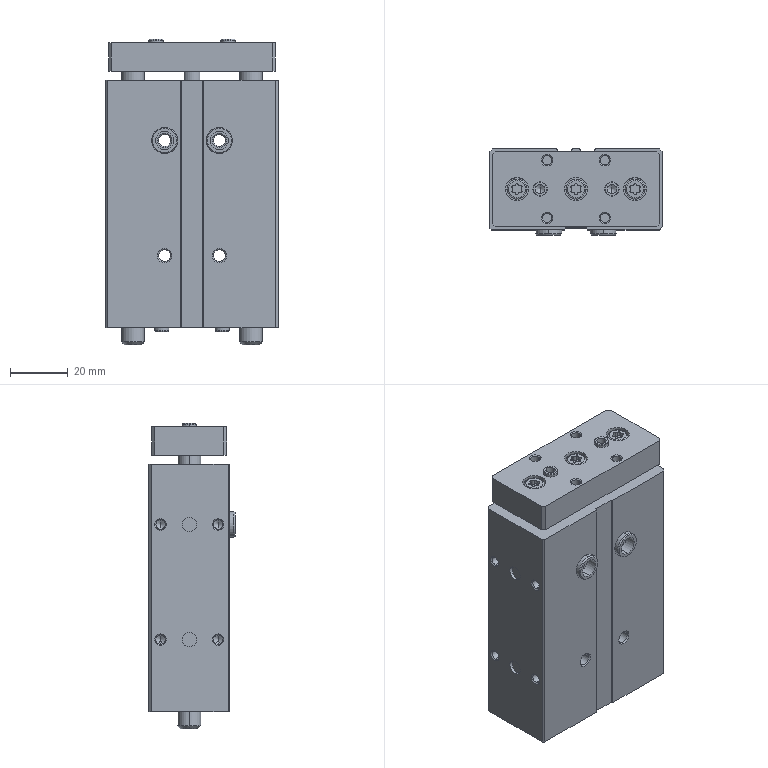Part | SolidWorks | 10 solids | 499 faces | box 60 x 29.95 x 106.2 mm | volume 146191 mm3 | cylinder 223 | plane 142 | cone 120 | spline 14 | commonest cylinder face diameters 5 x28 3.242 x26 8 x24 1.378 x21 0.4 x16 0.788 x16